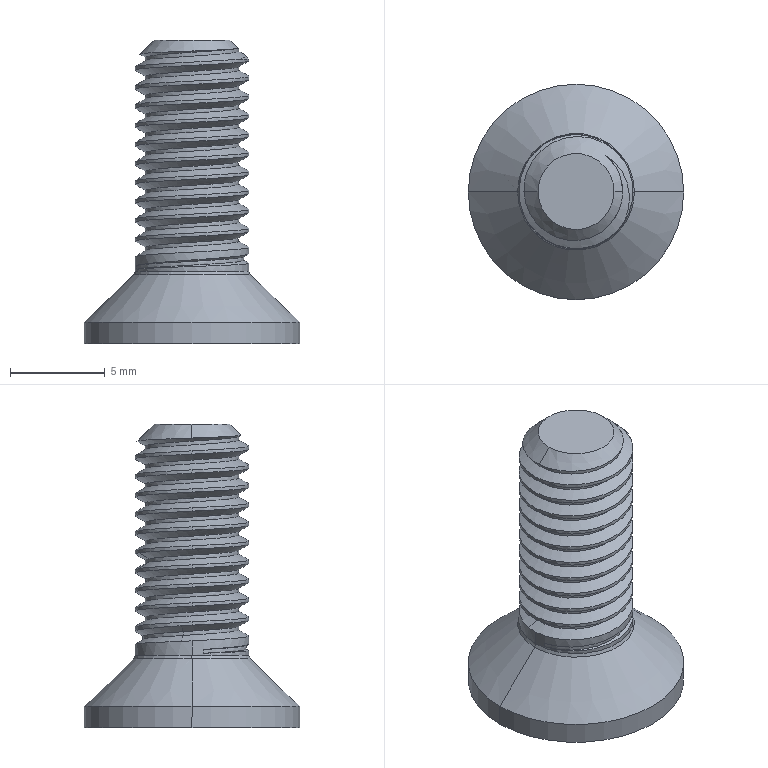Part | SolidWorks | features BaseBody 1 | 1 solid | 66 faces | box 11.34 x 11.34 x 16 mm | volume 524.212 mm3 | cylinder 25 | spline 14 | plane 14 | cone 13 | commonest cylinder face diameters 6 x23 11.34 x2